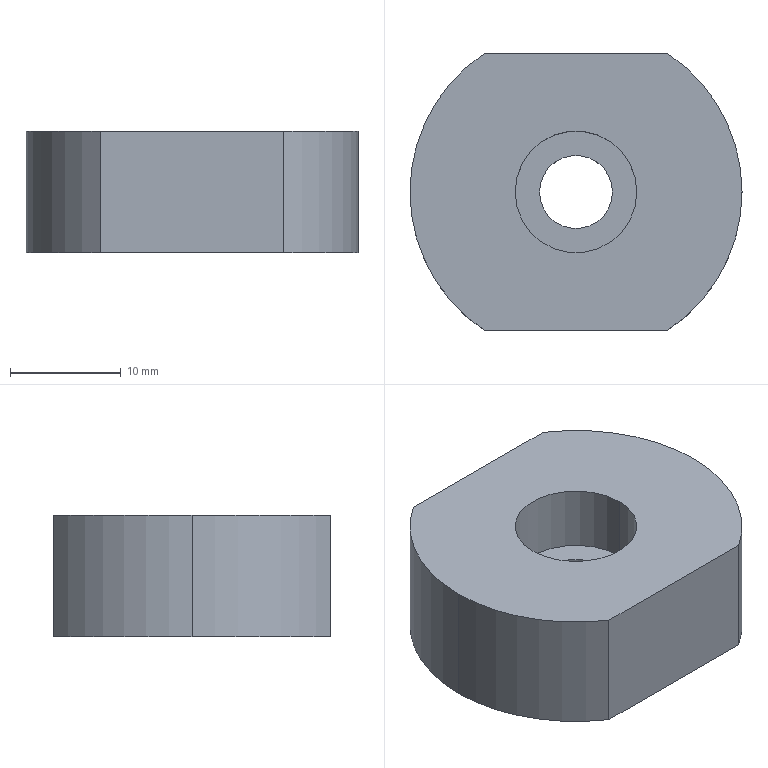Part | STEP file | union washer | 1 solid | 12 faces | box 30 x 25 x 11 mm | volume 6415 mm3 | cylinder 7 | plane 5 | commonest cylinder face diameters 30 x3 6.6 x2 11 x2
STEP:
#1=CARTESIAN_POINT('',(0.,0.,0.));
#2=DIRECTION('',(0.,0.,1.));
#3=DIRECTION('',(1.,0.,0.));
#4=AXIS2_PLACEMENT_3D('',#1,#2,#3);
#5=CARTESIAN_POINT('',(5.5,0.,5.));
#6=VERTEX_POINT('',#5);
#7=CARTESIAN_POINT('',(5.5,0.,11.));
#8=VERTEX_POINT('',#7);
#9=CARTESIAN_POINT('',(5.5,0.,11.));
#10=DIRECTION('',(0.,0.,1.));
#11=VECTOR('',#10,1.);
#12=LINE('',#9,#11);
#13=CARTESIAN_POINT('',(0.,0.,11.));
#14=DIRECTION('',(0.,0.,1.));
#15=DIRECTION('',(1.,0.,0.));
#16=AXIS2_PLACEMENT_3D('',#13,#14,#15);
#17=CYLINDRICAL_SURFACE('',#16,5.5);
#18=CARTESIAN_POINT('',(6.283,0.));
#19=DIRECTION('',(0.,1.));
#20=VECTOR('',#19,1.);
#21=LINE('',#18,#20);
#22=(GEOMETRIC_REPRESENTATION_CONTEXT(2)PARAMETRIC_REPRESENTATION_CONTEXT()REPRESENTATION_CONTEXT('',''));
#23=DEFINITIONAL_REPRESENTATION('',(#21),#22);
#24=PCURVE('',#17,#23);
#25=CARTESIAN_POINT('',(0.,0.,11.));
#26=DIRECTION('',(0.,0.,1.));
#27=DIRECTION('',(1.,0.,0.));
#28=AXIS2_PLACEMENT_3D('',#25,#26,#27);
#29=CYLINDRICAL_SURFACE('',#28,5.5);
#30=CARTESIAN_POINT('',(0.,0.));
#31=DIRECTION('',(0.,1.));
#32=VECTOR('',#31,1.);
#33=LINE('',#30,#32);
#34=(GEOMETRIC_REPRESENTATION_CONTEXT(2)PARAMETRIC_REPRESENTATION_CONTEXT()REPRESENTATION_CONTEXT('',''));
#35=DEFINITIONAL_REPRESENTATION('',(#33),#34);
#36=PCURVE('',#29,#35);
#37=SURFACE_CURVE('',#12,(#24,#36),.PCURVE_S1.);
#38=EDGE_CURVE('',#6,#8,#37,.T.);
#39=ORIENTED_EDGE('',*,*,#38,.T.);
#40=CARTESIAN_POINT('',(-5.5,0.,11.));
#41=VERTEX_POINT('',#40);
#42=CARTESIAN_POINT('',(0.,0.,11.));
#43=DIRECTION('',(0.,0.,1.));
#44=DIRECTION('',(1.,0.,0.));
#45=AXIS2_PLACEMENT_3D('',#42,#43,#44);
#46=CIRCLE('',#45,5.5);
#47=CARTESIAN_POINT('',(0.,0.));
#48=DIRECTION('',(1.,0.));
#49=VECTOR('',#48,1.);
#50=LINE('',#47,#49);
#51=(GEOMETRIC_REPRESENTATION_CONTEXT(2)PARAMETRIC_REPRESENTATION_CONTEXT()REPRESENTATION_CONTEXT('',''));
#52=DEFINITIONAL_REPRESENTATION('',(#50),#51);
#53=PCURVE('',#17,#52);
#54=CARTESIAN_POINT('',(0.,0.,11.));
#55=DIRECTION('',(0.,0.,1.));
#56=DIRECTION('',(1.,0.,0.));
#57=AXIS2_PLACEMENT_3D('',#54,#55,#56);
#58=PLANE('',#57);
#59=CARTESIAN_POINT('',(0.,0.));
#60=DIRECTION('',(1.,0.));
#61=AXIS2_PLACEMENT_2D('',#59,#60);
#62=CIRCLE('',#61,5.5);
#63=(GEOMETRIC_REPRESENTATION_CONTEXT(2)PARAMETRIC_REPRESENTATION_CONTEXT()REPRESENTATION_CONTEXT('',''));
#64=DEFINITIONAL_REPRESENTATION('',(#62),#63);
#65=PCURVE('',#58,#64);
#66=SURFACE_CURVE('',#46,(#53,#65),.PCURVE_S1.);
#67=EDGE_CURVE('',#41,#8,#66,.T.);
#68=ORIENTED_EDGE('',*,*,#67,.F.);
#69=CARTESIAN_POINT('',(-5.5,0.,5.));
#70=VERTEX_POINT('',#69);
#71=CARTESIAN_POINT('',(-5.5,0.,11.));
#72=DIRECTION('',(0.,0.,1.));
#73=VECTOR('',#72,1.);
#74=LINE('',#71,#73);
#75=CARTESIAN_POINT('',(3.142,0.));
#76=DIRECTION('',(0.,1.));
#77=VECTOR('',#76,1.);
#78=LINE('',#75,#77);
#79=(GEOMETRIC_REPRESENTATION_CONTEXT(2)PARAMETRIC_REPRESENTATION_CONTEXT()REPRESENTATION_CONTEXT('',''));
#80=DEFINITIONAL_REPRESENTATION('',(#78),#79);
#81=PCURVE('',#17,#80);
#82=CARTESIAN_POINT('',(3.142,0.));
#83=DIRECTION('',(0.,1.));
#84=VECTOR('',#83,1.);
#85=LINE('',#82,#84);
#86=(GEOMETRIC_REPRESENTATION_CONTEXT(2)PARAMETRIC_REPRESENTATION_CONTEXT()REPRESENTATION_CONTEXT('',''));
#87=DEFINITIONAL_REPRESENTATION('',(#85),#86);
#88=PCURVE('',#29,#87);
#89=SURFACE_CURVE('',#74,(#81,#88),.PCURVE_S1.);
#90=EDGE_CURVE('',#70,#41,#89,.T.);
#91=ORIENTED_EDGE('',*,*,#90,.F.);
#92=CARTESIAN_POINT('',(0.,0.,5.));
#93=DIRECTION('',(0.,0.,1.));
#94=DIRECTION('',(1.,0.,0.));
#95=AXIS2_PLACEMENT_3D('',#92,#93,#94);
#96=CIRCLE('',#95,5.5);
#97=CARTESIAN_POINT('',(0.,-6.));
#98=DIRECTION('',(1.,0.));
#99=VECTOR('',#98,1.);
#100=LINE('',#97,#99);
#101=(GEOMETRIC_REPRESENTATION_CONTEXT(2)PARAMETRIC_REPRESENTATION_CONTEXT()REPRESENTATION_CONTEXT('',''));
#102=DEFINITIONAL_REPRESENTATION('',(#100),#101);
#103=PCURVE('',#17,#102);
#104=CARTESIAN_POINT('',(3.3,0.,5.));
#105=DIRECTION('',(0.,0.,-1.));
#106=DIRECTION('',(-1.,0.,0.));
#107=AXIS2_PLACEMENT_3D('',#104,#105,#106);
#108=PLANE('',#107);
#109=CARTESIAN_POINT('',(-2.2,0.));
#110=CARTESIAN_POINT('',(-2.2,9.526));
#111=CARTESIAN_POINT('',(6.05,4.763));
#112=CARTESIAN_POINT('',(14.3,0.));
#113=CARTESIAN_POINT('',(6.05,-4.763));
#114=CARTESIAN_POINT('',(-2.2,-9.526));
#115=CARTESIAN_POINT('',(-2.2,0.));
#116=(BOUNDED_CURVE()B_SPLINE_CURVE(2,(#109,#110,#111,#112,#113,#114,#115),.UNSPECIFIED.,.T.,.F.)B_SPLINE_CURVE_WITH_KNOTS((1,2,2,2,2,1),(-2.094,0.,2.094,4.189,6.283,8.378),.UNSPECIFIED.)CURVE()GEOMETRIC_REPRESENTATION_ITEM()RATIONAL_B_SPLINE_CURVE((1.,0.5,1.,0.5,1.,0.5,1.))REPRESENTATION_ITEM(''));
#117=(GEOMETRIC_REPRESENTATION_CONTEXT(2)PARAMETRIC_REPRESENTATION_CONTEXT()REPRESENTATION_CONTEXT('',''));
#118=DEFINITIONAL_REPRESENTATION('',(#116),#117);
#119=PCURVE('',#108,#118);
#120=SURFACE_CURVE('',#96,(#103,#119),.PCURVE_S1.);
#121=EDGE_CURVE('',#70,#6,#120,.T.);
#122=ORIENTED_EDGE('',*,*,#121,.T.);
#123=EDGE_LOOP('',(#39,#68,#91,#122));
#124=FACE_BOUND('',#123,.F.);
#125=ADVANCED_FACE('',(#124),#17,.F.);
#126=CARTESIAN_POINT('',(-3.3,0.,5.));
#127=VERTEX_POINT('',#126);
#128=CARTESIAN_POINT('',(-3.3,0.,0.));
#129=VERTEX_POINT('',#128);
#130=CARTESIAN_POINT('',(-3.3,0.,11.));
#131=DIRECTION('',(0.,0.,-1.));
#132=VECTOR('',#131,1.);
#133=LINE('',#130,#132);
#134=CARTESIAN_POINT('',(0.,0.,11.));
#135=DIRECTION('',(0.,0.,-1.));
#136=DIRECTION('',(-1.,0.,0.));
#137=AXIS2_PLACEMENT_3D('',#134,#135,#136);
#138=CYLINDRICAL_SURFACE('',#137,3.3);
#139=CARTESIAN_POINT('',(6.283,0.));
#140=DIRECTION('',(0.,1.));
#141=VECTOR('',#140,1.);
#142=LINE('',#139,#141);
#143=(GEOMETRIC_REPRESENTATION_CONTEXT(2)PARAMETRIC_REPRESENTATION_CONTEXT()REPRESENTATION_CONTEXT('',''));
#144=DEFINITIONAL_REPRESENTATION('',(#142),#143);
#145=PCURVE('',#138,#144);
#146=CARTESIAN_POINT('',(0.,0.,11.));
#147=DIRECTION('',(0.,0.,-1.));
#148=DIRECTION('',(-1.,0.,0.));
#149=AXIS2_PLACEMENT_3D('',#146,#147,#148);
#150=CYLINDRICAL_SURFACE('',#149,3.3);
#151=CARTESIAN_POINT('',(0.,0.));
#152=DIRECTION('',(0.,1.));
#153=VECTOR('',#152,1.);
#154=LINE('',#151,#153);
#155=(GEOMETRIC_REPRESENTATION_CONTEXT(2)PARAMETRIC_REPRESENTATION_CONTEXT()REPRESENTATION_CONTEXT('',''));
#156=DEFINITIONAL_REPRESENTATION('',(#154),#155);
#157=PCURVE('',#150,#156);
#158=SURFACE_CURVE('',#133,(#145,#157),.PCURVE_S1.);
#159=EDGE_CURVE('',#127,#129,#158,.T.);
#160=ORIENTED_EDGE('',*,*,#159,.T.);
#161=CARTESIAN_POINT('',(3.3,0.,0.));
#162=VERTEX_POINT('',#161);
#163=CARTESIAN_POINT('',(0.,0.,0.));
#164=DIRECTION('',(0.,0.,1.));
#165=DIRECTION('',(1.,0.,0.));
#166=AXIS2_PLACEMENT_3D('',#163,#164,#165);
#167=CIRCLE('',#166,3.3);
#168=CARTESIAN_POINT('',(9.425,11.));
#169=DIRECTION('',(-1.,0.));
#170=VECTOR('',#169,1.);
#171=LINE('',#168,#170);
#172=(GEOMETRIC_REPRESENTATION_CONTEXT(2)PARAMETRIC_REPRESENTATION_CONTEXT()REPRESENTATION_CONTEXT('',''));
#173=DEFINITIONAL_REPRESENTATION('',(#171),#172);
#174=PCURVE('',#138,#173);
#175=CARTESIAN_POINT('',(0.,0.,0.));
#176=DIRECTION('',(0.,0.,1.));
#177=DIRECTION('',(1.,0.,0.));
#178=AXIS2_PLACEMENT_3D('',#175,#176,#177);
#179=PLANE('',#178);
#180=CARTESIAN_POINT('',(0.,0.));
#181=DIRECTION('',(1.,0.));
#182=AXIS2_PLACEMENT_2D('',#180,#181);
#183=CIRCLE('',#182,3.3);
#184=(GEOMETRIC_REPRESENTATION_CONTEXT(2)PARAMETRIC_REPRESENTATION_CONTEXT()REPRESENTATION_CONTEXT('',''));
#185=DEFINITIONAL_REPRESENTATION('',(#183),#184);
#186=PCURVE('',#179,#185);
#187=SURFACE_CURVE('',#167,(#174,#186),.PCURVE_S1.);
#188=EDGE_CURVE('',#129,#162,#187,.T.);
#189=ORIENTED_EDGE('',*,*,#188,.T.);
#190=CARTESIAN_POINT('',(3.3,0.,5.));
#191=VERTEX_POINT('',#190);
#192=CARTESIAN_POINT('',(3.3,0.,11.));
#193=DIRECTION('',(0.,0.,-1.));
#194=VECTOR('',#193,1.);
#195=LINE('',#192,#194);
#196=CARTESIAN_POINT('',(3.142,0.));
#197=DIRECTION('',(0.,1.));
#198=VECTOR('',#197,1.);
#199=LINE('',#196,#198);
#200=(GEOMETRIC_REPRESENTATION_CONTEXT(2)PARAMETRIC_REPRESENTATION_CONTEXT()REPRESENTATION_CONTEXT('',''));
#201=DEFINITIONAL_REPRESENTATION('',(#199),#200);
#202=PCURVE('',#138,#201);
#203=CARTESIAN_POINT('',(3.142,0.));
#204=DIRECTION('',(0.,1.));
#205=VECTOR('',#204,1.);
#206=LINE('',#203,#205);
#207=(GEOMETRIC_REPRESENTATION_CONTEXT(2)PARAMETRIC_REPRESENTATION_CONTEXT()REPRESENTATION_CONTEXT('',''));
#208=DEFINITIONAL_REPRESENTATION('',(#206),#207);
#209=PCURVE('',#150,#208);
#210=SURFACE_CURVE('',#195,(#202,#209),.PCURVE_S1.);
#211=EDGE_CURVE('',#191,#162,#210,.T.);
#212=ORIENTED_EDGE('',*,*,#211,.F.);
#213=CARTESIAN_POINT('',(0.,0.,5.));
#214=DIRECTION('',(0.,0.,1.));
#215=DIRECTION('',(1.,0.,0.));
#216=AXIS2_PLACEMENT_3D('',#213,#214,#215);
#217=CIRCLE('',#216,3.3);
#218=CARTESIAN_POINT('',(9.425,6.));
#219=DIRECTION('',(-1.,0.));
#220=VECTOR('',#219,1.);
#221=LINE('',#218,#220);
#222=(GEOMETRIC_REPRESENTATION_CONTEXT(2)PARAMETRIC_REPRESENTATION_CONTEXT()REPRESENTATION_CONTEXT('',''));
#223=DEFINITIONAL_REPRESENTATION('',(#221),#222);
#224=PCURVE('',#138,#223);
#225=CARTESIAN_POINT('',(0.,0.));
#226=CARTESIAN_POINT('',(0.,5.716));
#227=CARTESIAN_POINT('',(4.95,2.858));
#228=CARTESIAN_POINT('',(9.9,0.));
#229=CARTESIAN_POINT('',(4.95,-2.858));
#230=CARTESIAN_POINT('',(0.,-5.716));
#231=CARTESIAN_POINT('',(0.,0.));
#232=(BOUNDED_CURVE()B_SPLINE_CURVE(2,(#225,#226,#227,#228,#229,#230,#231),.UNSPECIFIED.,.T.,.F.)B_SPLINE_CURVE_WITH_KNOTS((1,2,2,2,2,1),(-2.094,0.,2.094,4.189,6.283,8.378),.UNSPECIFIED.)CURVE()GEOMETRIC_REPRESENTATION_ITEM()RATIONAL_B_SPLINE_CURVE((1.,0.5,1.,0.5,1.,0.5,1.))REPRESENTATION_ITEM(''));
#233=(GEOMETRIC_REPRESENTATION_CONTEXT(2)PARAMETRIC_REPRESENTATION_CONTEXT()REPRESENTATION_CONTEXT('',''));
#234=DEFINITIONAL_REPRESENTATION('',(#232),#233);
#235=PCURVE('',#108,#234);
#236=SURFACE_CURVE('',#217,(#224,#235),.PCURVE_S1.);
#237=EDGE_CURVE('',#127,#191,#236,.T.);
#238=ORIENTED_EDGE('',*,*,#237,.F.);
#239=EDGE_LOOP('',(#160,#189,#212,#238));
#240=FACE_BOUND('',#239,.F.);
#241=ADVANCED_FACE('',(#240),#138,.F.);
#242=CARTESIAN_POINT('',(-15.,0.,11.));
#243=VERTEX_POINT('',#242);
#244=CARTESIAN_POINT('',(-8.292,-12.5,11.));
#245=VERTEX_POINT('',#244);
#246=CARTESIAN_POINT('',(0.,0.,11.));
#247=DIRECTION('',(0.,0.,1.));
#248=DIRECTION('',(1.,0.,0.));
#249=AXIS2_PLACEMENT_3D('',#246,#247,#248);
#250=CIRCLE('',#249,15.);
#251=CARTESIAN_POINT('',(0.,0.,11.));
#252=DIRECTION('',(0.,0.,-1.));
#253=DIRECTION('',(-1.,0.,0.));
#254=AXIS2_PLACEMENT_3D('',#251,#252,#253);
#255=CYLINDRICAL_SURFACE('',#254,15.);
#256=CARTESIAN_POINT('',(9.425,0.));
#257=DIRECTION('',(-1.,0.));
#258=VECTOR('',#257,1.);
#259=LINE('',#256,#258);
#260=(GEOMETRIC_REPRESENTATION_CONTEXT(2)PARAMETRIC_REPRESENTATION_CONTEXT()REPRESENTATION_CONTEXT('',''));
#261=DEFINITIONAL_REPRESENTATION('',(#259),#260);
#262=PCURVE('',#255,#261);
#263=CARTESIAN_POINT('',(0.,0.));
#264=DIRECTION('',(1.,0.));
#265=AXIS2_PLACEMENT_2D('',#263,#264);
#266=CIRCLE('',#265,15.);
#267=(GEOMETRIC_REPRESENTATION_CONTEXT(2)PARAMETRIC_REPRESENTATION_CONTEXT()REPRESENTATION_CONTEXT('',''));
#268=DEFINITIONAL_REPRESENTATION('',(#266),#267);
#269=PCURVE('',#58,#268);
#270=SURFACE_CURVE('',#250,(#262,#269),.PCURVE_S1.);
#271=EDGE_CURVE('',#243,#245,#270,.T.);
#272=ORIENTED_EDGE('',*,*,#271,.F.);
#273=CARTESIAN_POINT('',(-15.,0.,0.));
#274=VERTEX_POINT('',#273);
#275=CARTESIAN_POINT('',(-15.,0.,11.));
#276=DIRECTION('',(0.,0.,-1.));
#277=VECTOR('',#276,1.);
#278=LINE('',#275,#277);
#279=CARTESIAN_POINT('',(6.283,0.));
#280=DIRECTION('',(0.,1.));
#281=VECTOR('',#280,1.);
#282=LINE('',#279,#281);
#283=(GEOMETRIC_REPRESENTATION_CONTEXT(2)PARAMETRIC_REPRESENTATION_CONTEXT()REPRESENTATION_CONTEXT('',''));
#284=DEFINITIONAL_REPRESENTATION('',(#282),#283);
#285=PCURVE('',#255,#284);
#286=CARTESIAN_POINT('',(0.,0.,11.));
#287=DIRECTION('',(0.,0.,-1.));
#288=DIRECTION('',(-1.,0.,0.));
#289=AXIS2_PLACEMENT_3D('',#286,#287,#288);
#290=CYLINDRICAL_SURFACE('',#289,15.);
#291=CARTESIAN_POINT('',(0.,0.));
#292=DIRECTION('',(0.,1.));
#293=VECTOR('',#292,1.);
#294=LINE('',#291,#293);
#295=(GEOMETRIC_REPRESENTATION_CONTEXT(2)PARAMETRIC_REPRESENTATION_CONTEXT()REPRESENTATION_CONTEXT('',''));
#296=DEFINITIONAL_REPRESENTATION('',(#294),#295);
#297=PCURVE('',#290,#296);
#298=SURFACE_CURVE('',#278,(#285,#297),.PCURVE_S1.);
#299=EDGE_CURVE('',#243,#274,#298,.T.);
#300=ORIENTED_EDGE('',*,*,#299,.T.);
#301=CARTESIAN_POINT('',(-8.292,-12.5,0.));
#302=VERTEX_POINT('',#301);
#303=CARTESIAN_POINT('',(0.,0.,0.));
#304=DIRECTION('',(0.,0.,1.));
#305=DIRECTION('',(1.,0.,0.));
#306=AXIS2_PLACEMENT_3D('',#303,#304,#305);
#307=CIRCLE('',#306,15.);
#308=CARTESIAN_POINT('',(9.425,11.));
#309=DIRECTION('',(-1.,0.));
#310=VECTOR('',#309,1.);
#311=LINE('',#308,#310);
#312=(GEOMETRIC_REPRESENTATION_CONTEXT(2)PARAMETRIC_REPRESENTATION_CONTEXT()REPRESENTATION_CONTEXT('',''));
#313=DEFINITIONAL_REPRESENTATION('',(#311),#312);
#314=PCURVE('',#255,#313);
#315=CARTESIAN_POINT('',(0.,0.));
#316=DIRECTION('',(1.,0.));
#317=AXIS2_PLACEMENT_2D('',#315,#316);
#318=CIRCLE('',#317,15.);
#319=(GEOMETRIC_REPRESENTATION_CONTEXT(2)PARAMETRIC_REPRESENTATION_CONTEXT()REPRESENTATION_CONTEXT('',''));
#320=DEFINITIONAL_REPRESENTATION('',(#318),#319);
#321=PCURVE('',#179,#320);
#322=SURFACE_CURVE('',#307,(#314,#321),.PCURVE_S1.);
#323=EDGE_CURVE('',#274,#302,#322,.T.);
#324=ORIENTED_EDGE('',*,*,#323,.T.);
#325=CARTESIAN_POINT('',(-8.292,-12.5,11.));
#326=DIRECTION('',(0.,0.,-1.));
#327=VECTOR('',#326,1.);
#328=LINE('',#325,#327);
#329=CARTESIAN_POINT('',(5.298,0.));
#330=DIRECTION('',(0.,1.));
#331=VECTOR('',#330,1.);
#332=LINE('',#329,#331);
#333=(GEOMETRIC_REPRESENTATION_CONTEXT(2)PARAMETRIC_REPRESENTATION_CONTEXT()REPRESENTATION_CONTEXT('',''));
#334=DEFINITIONAL_REPRESENTATION('',(#332),#333);
#335=PCURVE('',#255,#334);
#336=CARTESIAN_POINT('',(-8.292,-12.5,11.));
#337=DIRECTION('',(0.,1.,0.));
#338=DIRECTION('',(0.,0.,1.));
#339=AXIS2_PLACEMENT_3D('',#336,#337,#338);
#340=PLANE('',#339);
#341=CARTESIAN_POINT('',(0.,0.));
#342=DIRECTION('',(-1.,0.));
#343=VECTOR('',#342,1.);
#344=LINE('',#341,#343);
#345=(GEOMETRIC_REPRESENTATION_CONTEXT(2)PARAMETRIC_REPRESENTATION_CONTEXT()REPRESENTATION_CONTEXT('',''));
#346=DEFINITIONAL_REPRESENTATION('',(#344),#345);
#347=PCURVE('',#340,#346);
#348=SURFACE_CURVE('',#328,(#335,#347),.PCURVE_S1.);
#349=EDGE_CURVE('',#245,#302,#348,.T.);
#350=ORIENTED_EDGE('',*,*,#349,.F.);
#351=EDGE_LOOP('',(#272,#300,#324,#350));
#352=FACE_BOUND('',#351,.T.);
#353=ADVANCED_FACE('',(#352),#255,.T.);
#354=CARTESIAN_POINT('',(0.,0.,11.));
#355=DIRECTION('',(0.,0.,1.));
#356=DIRECTION('',(1.,0.,0.));
#357=AXIS2_PLACEMENT_3D('',#354,#355,#356);
#358=CIRCLE('',#357,5.5);
#359=CARTESIAN_POINT('',(0.,0.));
#360=DIRECTION('',(1.,0.));
#361=AXIS2_PLACEMENT_2D('',#359,#360);
#362=CIRCLE('',#361,5.5);
#363=(GEOMETRIC_REPRESENTATION_CONTEXT(2)PARAMETRIC_REPRESENTATION_CONTEXT()REPRESENTATION_CONTEXT('',''));
#364=DEFINITIONAL_REPRESENTATION('',(#362),#363);
#365=PCURVE('',#58,#364);
#366=CARTESIAN_POINT('',(0.,0.));
#367=DIRECTION('',(1.,0.));
#368=VECTOR('',#367,1.);
#369=LINE('',#366,#368);
#370=(GEOMETRIC_REPRESENTATION_CONTEXT(2)PARAMETRIC_REPRESENTATION_CONTEXT()REPRESENTATION_CONTEXT('',''));
#371=DEFINITIONAL_REPRESENTATION('',(#369),#370);
#372=PCURVE('',#29,#371);
#373=SURFACE_CURVE('',#358,(#365,#372),.PCURVE_S1.);
#374=EDGE_CURVE('',#8,#41,#373,.T.);
#375=ORIENTED_EDGE('',*,*,#374,.F.);
#376=ORIENTED_EDGE('',*,*,#67,.F.);
#377=EDGE_LOOP('',(#375,#376));
#378=FACE_BOUND('',#377,.T.);
#379=CARTESIAN_POINT('',(-8.292,12.5,11.));
#380=VERTEX_POINT('',#379);
#381=CARTESIAN_POINT('',(0.,0.,11.));
#382=DIRECTION('',(0.,0.,1.));
#383=DIRECTION('',(1.,0.,0.));
#384=AXIS2_PLACEMENT_3D('',#381,#382,#383);
#385=CIRCLE('',#384,15.);
#386=CARTESIAN_POINT('',(0.,0.));
#387=DIRECTION('',(1.,0.));
#388=AXIS2_PLACEMENT_2D('',#386,#387);
#389=CIRCLE('',#388,15.);
#390=(GEOMETRIC_REPRESENTATION_CONTEXT(2)PARAMETRIC_REPRESENTATION_CONTEXT()REPRESENTATION_CONTEXT('',''));
#391=DEFINITIONAL_REPRESENTATION('',(#389),#390);
#392=PCURVE('',#58,#391);
#393=CARTESIAN_POINT('',(3.142,0.));
#394=DIRECTION('',(-1.,0.));
#395=VECTOR('',#394,1.);
#396=LINE('',#393,#395);
#397=(GEOMETRIC_REPRESENTATION_CONTEXT(2)PARAMETRIC_REPRESENTATION_CONTEXT()REPRESENTATION_CONTEXT('',''));
#398=DEFINITIONAL_REPRESENTATION('',(#396),#397);
#399=PCURVE('',#290,#398);
#400=SURFACE_CURVE('',#385,(#392,#399),.PCURVE_S1.);
#401=EDGE_CURVE('',#380,#243,#400,.T.);
#402=ORIENTED_EDGE('',*,*,#401,.T.);
#403=ORIENTED_EDGE('',*,*,#271,.T.);
#404=CARTESIAN_POINT('',(8.292,-12.5,11.));
#405=VERTEX_POINT('',#404);
#406=CARTESIAN_POINT('',(-8.292,-12.5,11.));
#407=DIRECTION('',(1.,0.,0.));
#408=VECTOR('',#407,1.);
#409=LINE('',#406,#408);
#410=CARTESIAN_POINT('',(-8.292,-12.5));
#411=DIRECTION('',(1.,0.));
#412=VECTOR('',#411,1.);
#413=LINE('',#410,#412);
#414=(GEOMETRIC_REPRESENTATION_CONTEXT(2)PARAMETRIC_REPRESENTATION_CONTEXT()REPRESENTATION_CONTEXT('',''));
#415=DEFINITIONAL_REPRESENTATION('',(#413),#414);
#416=PCURVE('',#58,#415);
#417=CARTESIAN_POINT('',(0.,0.));
#418=DIRECTION('',(0.,1.));
#419=VECTOR('',#418,1.);
#420=LINE('',#417,#419);
#421=(GEOMETRIC_REPRESENTATION_CONTEXT(2)PARAMETRIC_REPRESENTATION_CONTEXT()REPRESENTATION_CONTEXT('',''));
#422=DEFINITIONAL_REPRESENTATION('',(#420),#421);
#423=PCURVE('',#340,#422);
#424=SURFACE_CURVE('',#409,(#416,#423),.PCURVE_S1.);
#425=EDGE_CURVE('',#245,#405,#424,.T.);
#426=ORIENTED_EDGE('',*,*,#425,.T.);
#427=CARTESIAN_POINT('',(8.292,12.5,11.));
#428=VERTEX_POINT('',#427);
#429=CARTESIAN_POINT('',(0.,0.,11.));
#430=DIRECTION('',(0.,0.,1.));
#431=DIRECTION('',(1.,0.,0.));
#432=AXIS2_PLACEMENT_3D('',#429,#430,#431);
#433=CIRCLE('',#432,15.);
#434=CARTESIAN_POINT('',(0.,0.));
#435=DIRECTION('',(1.,0.));
#436=AXIS2_PLACEMENT_2D('',#434,#435);
#437=CIRCLE('',#436,15.);
#438=(GEOMETRIC_REPRESENTATION_CONTEXT(2)PARAMETRIC_REPRESENTATION_CONTEXT()REPRESENTATION_CONTEXT('',''));
#439=DEFINITIONAL_REPRESENTATION('',(#437),#438);
#440=PCURVE('',#58,#439);
#441=CARTESIAN_POINT('',(0.,0.,11.));
#442=DIRECTION('',(0.,0.,-1.));
#443=DIRECTION('',(-1.,0.,0.));
#444=AXIS2_PLACEMENT_3D('',#441,#442,#443);
#445=CYLINDRICAL_SURFACE('',#444,15.);
#446=CARTESIAN_POINT('',(9.425,0.));
#447=DIRECTION('',(-1.,0.));
#448=VECTOR('',#447,1.);
#449=LINE('',#446,#448);
#450=(GEOMETRIC_REPRESENTATION_CONTEXT(2)PARAMETRIC_REPRESENTATION_CONTEXT()REPRESENTATION_CONTEXT('',''));
#451=DEFINITIONAL_REPRESENTATION('',(#449),#450);
#452=PCURVE('',#445,#451);
#453=SURFACE_CURVE('',#433,(#440,#452),.PCURVE_S1.);
#454=EDGE_CURVE('',#405,#428,#453,.T.);
#455=ORIENTED_EDGE('',*,*,#454,.T.);
#456=CARTESIAN_POINT('',(8.292,12.5,11.));
#457=DIRECTION('',(-1.,0.,0.));
#458=VECTOR('',#457,1.);
#459=LINE('',#456,#458);
#460=CARTESIAN_POINT('',(8.292,12.5));
#461=DIRECTION('',(-1.,0.));
#462=VECTOR('',#461,1.);
#463=LINE('',#460,#462);
#464=(GEOMETRIC_REPRESENTATION_CONTEXT(2)PARAMETRIC_REPRESENTATION_CONTEXT()REPRESENTATION_CONTEXT('',''));
#465=DEFINITIONAL_REPRESENTATION('',(#463),#464);
#466=PCURVE('',#58,#465);
#467=CARTESIAN_POINT('',(8.292,12.5,11.));
#468=DIRECTION('',(0.,-1.,0.));
#469=DIRECTION('',(0.,0.,-1.));
#470=AXIS2_PLACEMENT_3D('',#467,#468,#469);
#471=PLANE('',#470);
#472=CARTESIAN_POINT('',(0.,0.));
#473=DIRECTION('',(0.,-1.));
#474=VECTOR('',#473,1.);
#475=LINE('',#472,#474);
#476=(GEOMETRIC_REPRESENTATION_CONTEXT(2)PARAMETRIC_REPRESENTATION_CONTEXT()REPRESENTATION_CONTEXT('',''));
#477=DEFINITIONAL_REPRESENTATION('',(#475),#476);
#478=PCURVE('',#471,#477);
#479=SURFACE_CURVE('',#459,(#466,#478),.PCURVE_S1.);
#480=EDGE_CURVE('',#428,#380,#479,.T.);
#481=ORIENTED_EDGE('',*,*,#480,.T.);
#482=EDGE_LOOP('',(#402,#403,#426,#455,#481));
#483=FACE_BOUND('',#482,.T.);
#484=ADVANCED_FACE('',(#378,#483),#58,.T.);
#485=CARTESIAN_POINT('',(-8.292,12.5,0.));
#486=VERTEX_POINT('',#485);
#487=CARTESIAN_POINT('',(0.,0.,0.));
#488=DIRECTION('',(0.,0.,1.));
#489=DIRECTION('',(1.,0.,0.));
#490=AXIS2_PLACEMENT_3D('',#487,#488,#489);
#491=CIRCLE('',#490,15.);
#492=CARTESIAN_POINT('',(0.,0.));
#493=DIRECTION('',(1.,0.));
#494=AXIS2_PLACEMENT_2D('',#492,#493);
#495=CIRCLE('',#494,15.);
#496=(GEOMETRIC_REPRESENTATION_CONTEXT(2)PARAMETRIC_REPRESENTATION_CONTEXT()REPRESENTATION_CONTEXT('',''));
#497=DEFINITIONAL_REPRESENTATION('',(#495),#496);
#498=PCURVE('',#179,#497);
#499=CARTESIAN_POINT('',(3.142,11.));
#500=DIRECTION('',(-1.,0.));
#501=VECTOR('',#500,1.);
#502=LINE('',#499,#501);
#503=(GEOMETRIC_REPRESENTATION_CONTEXT(2)PARAMETRIC_REPRESENTATION_CONTEXT()REPRESENTATION_CONTEXT('',''));
#504=DEFINITIONAL_REPRESENTATION('',(#502),#503);
#505=PCURVE('',#290,#504);
#506=SURFACE_CURVE('',#491,(#498,#505),.PCURVE_S1.);
#507=EDGE_CURVE('',#486,#274,#506,.T.);
#508=ORIENTED_EDGE('',*,*,#507,.F.);
#509=CARTESIAN_POINT('',(8.292,12.5,0.));
#510=VERTEX_POINT('',#509);
#511=CARTESIAN_POINT('',(8.292,12.5,0.));
#512=DIRECTION('',(-1.,0.,0.));
#513=VECTOR('',#512,1.);
#514=LINE('',#511,#513);
#515=CARTESIAN_POINT('',(8.292,12.5));
#516=DIRECTION('',(-1.,0.));
#517=VECTOR('',#516,1.);
#518=LINE('',#515,#517);
#519=(GEOMETRIC_REPRESENTATION_CONTEXT(2)PARAMETRIC_REPRESENTATION_CONTEXT()REPRESENTATION_CONTEXT('',''));
#520=DEFINITIONAL_REPRESENTATION('',(#518),#519);
#521=PCURVE('',#179,#520);
#522=CARTESIAN_POINT('',(11.,0.));
#523=DIRECTION('',(0.,-1.));
#524=VECTOR('',#523,1.);
#525=LINE('',#522,#524);
#526=(GEOMETRIC_REPRESENTATION_CONTEXT(2)PARAMETRIC_REPRESENTATION_CONTEXT()REPRESENTATION_CONTEXT('',''));
#527=DEFINITIONAL_REPRESENTATION('',(#525),#526);
#528=PCURVE('',#471,#527);
#529=SURFACE_CURVE('',#514,(#521,#528),.PCURVE_S1.);
#530=EDGE_CURVE('',#510,#486,#529,.T.);
#531=ORIENTED_EDGE('',*,*,#530,.F.);
#532=CARTESIAN_POINT('',(8.292,-12.5,0.));
#533=VERTEX_POINT('',#532);
#534=CARTESIAN_POINT('',(0.,0.,0.));
#535=DIRECTION('',(0.,0.,1.));
#536=DIRECTION('',(1.,0.,0.));
#537=AXIS2_PLACEMENT_3D('',#534,#535,#536);
#538=CIRCLE('',#537,15.);
#539=CARTESIAN_POINT('',(0.,0.));
#540=DIRECTION('',(1.,0.));
#541=AXIS2_PLACEMENT_2D('',#539,#540);
#542=CIRCLE('',#541,15.);
#543=(GEOMETRIC_REPRESENTATION_CONTEXT(2)PARAMETRIC_REPRESENTATION_CONTEXT()REPRESENTATION_CONTEXT('',''));
#544=DEFINITIONAL_REPRESENTATION('',(#542),#543);
#545=PCURVE('',#179,#544);
#546=CARTESIAN_POINT('',(9.425,11.));
#547=DIRECTION('',(-1.,0.));
#548=VECTOR('',#547,1.);
#549=LINE('',#546,#548);
#550=(GEOMETRIC_REPRESENTATION_CONTEXT(2)PARAMETRIC_REPRESENTATION_CONTEXT()REPRESENTATION_CONTEXT('',''));
#551=DEFINITIONAL_REPRESENTATION('',(#549),#550);
#552=PCURVE('',#445,#551);
#553=SURFACE_CURVE('',#538,(#545,#552),.PCURVE_S1.);
#554=EDGE_CURVE('',#533,#510,#553,.T.);
#555=ORIENTED_EDGE('',*,*,#554,.F.);
#556=CARTESIAN_POINT('',(-8.292,-12.5,0.));
#557=DIRECTION('',(1.,0.,0.));
#558=VECTOR('',#557,1.);
#559=LINE('',#556,#558);
#560=CARTESIAN_POINT('',(-8.292,-12.5));
#561=DIRECTION('',(1.,0.));
#562=VECTOR('',#561,1.);
#563=LINE('',#560,#562);
#564=(GEOMETRIC_REPRESENTATION_CONTEXT(2)PARAMETRIC_REPRESENTATION_CONTEXT()REPRESENTATION_CONTEXT('',''));
#565=DEFINITIONAL_REPRESENTATION('',(#563),#564);
#566=PCURVE('',#179,#565);
#567=CARTESIAN_POINT('',(-11.,0.));
#568=DIRECTION('',(0.,1.));
#569=VECTOR('',#568,1.);
#570=LINE('',#567,#569);
#571=(GEOMETRIC_REPRESENTATION_CONTEXT(2)PARAMETRIC_REPRESENTATION_CONTEXT()REPRESENTATION_CONTEXT('',''));
#572=DEFINITIONAL_REPRESENTATION('',(#570),#571);
#573=PCURVE('',#340,#572);
#574=SURFACE_CURVE('',#559,(#566,#573),.PCURVE_S1.);
#575=EDGE_CURVE('',#302,#533,#574,.T.);
#576=ORIENTED_EDGE('',*,*,#575,.F.);
#577=ORIENTED_EDGE('',*,*,#323,.F.);
#578=EDGE_LOOP('',(#508,#531,#555,#576,#577));
#579=FACE_BOUND('',#578,.T.);
#580=ORIENTED_EDGE('',*,*,#188,.T.);
#581=CARTESIAN_POINT('',(0.,0.,0.));
#582=DIRECTION('',(0.,0.,1.));
#583=DIRECTION('',(1.,0.,0.));
#584=AXIS2_PLACEMENT_3D('',#581,#582,#583);
#585=CIRCLE('',#584,3.3);
#586=CARTESIAN_POINT('',(0.,0.));
#587=DIRECTION('',(1.,0.));
#588=AXIS2_PLACEMENT_2D('',#586,#587);
#589=CIRCLE('',#588,3.3);
#590=(GEOMETRIC_REPRESENTATION_CONTEXT(2)PARAMETRIC_REPRESENTATION_CONTEXT()REPRESENTATION_CONTEXT('',''));
#591=DEFINITIONAL_REPRESENTATION('',(#589),#590);
#592=PCURVE('',#179,#591);
#593=CARTESIAN_POINT('',(3.142,11.));
#594=DIRECTION('',(-1.,0.));
#595=VECTOR('',#594,1.);
#596=LINE('',#593,#595);
#597=(GEOMETRIC_REPRESENTATION_CONTEXT(2)PARAMETRIC_REPRESENTATION_CONTEXT()REPRESENTATION_CONTEXT('',''));
#598=DEFINITIONAL_REPRESENTATION('',(#596),#597);
#599=PCURVE('',#150,#598);
#600=SURFACE_CURVE('',#585,(#592,#599),.PCURVE_S1.);
#601=EDGE_CURVE('',#162,#129,#600,.T.);
#602=ORIENTED_EDGE('',*,*,#601,.T.);
#603=EDGE_LOOP('',(#580,#602));
#604=FACE_BOUND('',#603,.T.);
#605=ADVANCED_FACE('',(#579,#604),#179,.F.);
#606=ORIENTED_EDGE('',*,*,#299,.F.);
#607=ORIENTED_EDGE('',*,*,#401,.F.);
#608=CARTESIAN_POINT('',(-8.292,12.5,11.));
#609=DIRECTION('',(0.,0.,-1.));
#610=VECTOR('',#609,1.);
#611=LINE('',#608,#610);
#612=CARTESIAN_POINT('',(0.9851,0.));
#613=DIRECTION('',(0.,1.));
#614=VECTOR('',#613,1.);
#615=LINE('',#612,#614);
#616=(GEOMETRIC_REPRESENTATION_CONTEXT(2)PARAMETRIC_REPRESENTATION_CONTEXT()REPRESENTATION_CONTEXT('',''));
#617=DEFINITIONAL_REPRESENTATION('',(#615),#616);
#618=PCURVE('',#290,#617);
#619=CARTESIAN_POINT('',(0.,-16.583));
#620=DIRECTION('',(1.,0.));
#621=VECTOR('',#620,1.);
#622=LINE('',#619,#621);
#623=(GEOMETRIC_REPRESENTATION_CONTEXT(2)PARAMETRIC_REPRESENTATION_CONTEXT()REPRESENTATION_CONTEXT('',''));
#624=DEFINITIONAL_REPRESENTATION('',(#622),#623);
#625=PCURVE('',#471,#624);
#626=SURFACE_CURVE('',#611,(#618,#625),.PCURVE_S1.);
#627=EDGE_CURVE('',#380,#486,#626,.T.);
#628=ORIENTED_EDGE('',*,*,#627,.T.);
#629=ORIENTED_EDGE('',*,*,#507,.T.);
#630=EDGE_LOOP('',(#606,#607,#628,#629));
#631=FACE_BOUND('',#630,.T.);
#632=ADVANCED_FACE('',(#631),#290,.T.);
#633=ORIENTED_EDGE('',*,*,#575,.T.);
#634=CARTESIAN_POINT('',(8.292,-12.5,11.));
#635=DIRECTION('',(0.,0.,-1.));
#636=VECTOR('',#635,1.);
#637=LINE('',#634,#636);
#638=CARTESIAN_POINT('',(0.,16.583));
#639=DIRECTION('',(-1.,0.));
#640=VECTOR('',#639,1.);
#641=LINE('',#638,#640);
#642=(GEOMETRIC_REPRESENTATION_CONTEXT(2)PARAMETRIC_REPRESENTATION_CONTEXT()REPRESENTATION_CONTEXT('',''));
#643=DEFINITIONAL_REPRESENTATION('',(#641),#642);
#644=PCURVE('',#340,#643);
#645=CARTESIAN_POINT('',(4.127,0.));
#646=DIRECTION('',(0.,1.));
#647=VECTOR('',#646,1.);
#648=LINE('',#645,#647);
#649=(GEOMETRIC_REPRESENTATION_CONTEXT(2)PARAMETRIC_REPRESENTATION_CONTEXT()REPRESENTATION_CONTEXT('',''));
#650=DEFINITIONAL_REPRESENTATION('',(#648),#649);
#651=PCURVE('',#445,#650);
#652=SURFACE_CURVE('',#637,(#644,#651),.PCURVE_S1.);
#653=EDGE_CURVE('',#405,#533,#652,.T.);
#654=ORIENTED_EDGE('',*,*,#653,.F.);
#655=ORIENTED_EDGE('',*,*,#425,.F.);
#656=ORIENTED_EDGE('',*,*,#349,.T.);
#657=EDGE_LOOP('',(#633,#654,#655,#656));
#658=FACE_BOUND('',#657,.T.);
#659=ADVANCED_FACE('',(#658),#340,.F.);
#660=ORIENTED_EDGE('',*,*,#554,.T.);
#661=CARTESIAN_POINT('',(8.292,12.5,11.));
#662=DIRECTION('',(0.,0.,-1.));
#663=VECTOR('',#662,1.);
#664=LINE('',#661,#663);
#665=CARTESIAN_POINT('',(2.156,0.));
#666=DIRECTION('',(0.,1.));
#667=VECTOR('',#666,1.);
#668=LINE('',#665,#667);
#669=(GEOMETRIC_REPRESENTATION_CONTEXT(2)PARAMETRIC_REPRESENTATION_CONTEXT()REPRESENTATION_CONTEXT('',''));
#670=DEFINITIONAL_REPRESENTATION('',(#668),#669);
#671=PCURVE('',#445,#670);
#672=CARTESIAN_POINT('',(0.,0.));
#673=DIRECTION('',(1.,0.));
#674=VECTOR('',#673,1.);
#675=LINE('',#672,#674);
#676=(GEOMETRIC_REPRESENTATION_CONTEXT(2)PARAMETRIC_REPRESENTATION_CONTEXT()REPRESENTATION_CONTEXT('',''));
#677=DEFINITIONAL_REPRESENTATION('',(#675),#676);
#678=PCURVE('',#471,#677);
#679=SURFACE_CURVE('',#664,(#671,#678),.PCURVE_S1.);
#680=EDGE_CURVE('',#428,#510,#679,.T.);
#681=ORIENTED_EDGE('',*,*,#680,.F.);
#682=ORIENTED_EDGE('',*,*,#454,.F.);
#683=ORIENTED_EDGE('',*,*,#653,.T.);
#684=EDGE_LOOP('',(#660,#681,#682,#683));
#685=FACE_BOUND('',#684,.T.);
#686=ADVANCED_FACE('',(#685),#445,.T.);
#687=ORIENTED_EDGE('',*,*,#530,.T.);
#688=ORIENTED_EDGE('',*,*,#627,.F.);
#689=ORIENTED_EDGE('',*,*,#480,.F.);
#690=ORIENTED_EDGE('',*,*,#680,.T.);
#691=EDGE_LOOP('',(#687,#688,#689,#690));
#692=FACE_BOUND('',#691,.T.);
#693=ADVANCED_FACE('',(#692),#471,.F.);
#694=ORIENTED_EDGE('',*,*,#601,.T.);
#695=ORIENTED_EDGE('',*,*,#159,.F.);
#696=CARTESIAN_POINT('',(0.,0.,5.));
#697=DIRECTION('',(0.,0.,1.));
#698=DIRECTION('',(1.,0.,0.));
#699=AXIS2_PLACEMENT_3D('',#696,#697,#698);
#700=CIRCLE('',#699,3.3);
#701=CARTESIAN_POINT('',(3.142,6.));
#702=DIRECTION('',(-1.,0.));
#703=VECTOR('',#702,1.);
#704=LINE('',#701,#703);
#705=(GEOMETRIC_REPRESENTATION_CONTEXT(2)PARAMETRIC_REPRESENTATION_CONTEXT()REPRESENTATION_CONTEXT('',''));
#706=DEFINITIONAL_REPRESENTATION('',(#704),#705);
#707=PCURVE('',#150,#706);
#708=CARTESIAN_POINT('',(0.,0.));
#709=CARTESIAN_POINT('',(0.,5.716));
#710=CARTESIAN_POINT('',(4.95,2.858));
#711=CARTESIAN_POINT('',(9.9,0.));
#712=CARTESIAN_POINT('',(4.95,-2.858));
#713=CARTESIAN_POINT('',(0.,-5.716));
#714=CARTESIAN_POINT('',(0.,0.));
#715=(BOUNDED_CURVE()B_SPLINE_CURVE(2,(#708,#709,#710,#711,#712,#713,#714),.UNSPECIFIED.,.T.,.F.)B_SPLINE_CURVE_WITH_KNOTS((1,2,2,2,2,1),(-2.094,0.,2.094,4.189,6.283,8.378),.UNSPECIFIED.)CURVE()GEOMETRIC_REPRESENTATION_ITEM()RATIONAL_B_SPLINE_CURVE((1.,0.5,1.,0.5,1.,0.5,1.))REPRESENTATION_ITEM(''));
#716=(GEOMETRIC_REPRESENTATION_CONTEXT(2)PARAMETRIC_REPRESENTATION_CONTEXT()REPRESENTATION_CONTEXT('',''));
#717=DEFINITIONAL_REPRESENTATION('',(#715),#716);
#718=PCURVE('',#108,#717);
#719=SURFACE_CURVE('',#700,(#707,#718),.PCURVE_S1.);
#720=EDGE_CURVE('',#191,#127,#719,.T.);
#721=ORIENTED_EDGE('',*,*,#720,.F.);
#722=ORIENTED_EDGE('',*,*,#211,.T.);
#723=EDGE_LOOP('',(#694,#695,#721,#722));
#724=FACE_BOUND('',#723,.F.);
#725=ADVANCED_FACE('',(#724),#150,.F.);
#726=ORIENTED_EDGE('',*,*,#237,.F.);
#727=ORIENTED_EDGE('',*,*,#720,.F.);
#728=EDGE_LOOP('',(#726,#727));
#729=FACE_BOUND('',#728,.T.);
#730=CARTESIAN_POINT('',(0.,0.,5.));
#731=DIRECTION('',(0.,0.,1.));
#732=DIRECTION('',(1.,0.,0.));
#733=AXIS2_PLACEMENT_3D('',#730,#731,#732);
#734=CIRCLE('',#733,5.5);
#735=CARTESIAN_POINT('',(-2.2,0.));
#736=CARTESIAN_POINT('',(-2.2,9.526));
#737=CARTESIAN_POINT('',(6.05,4.763));
#738=CARTESIAN_POINT('',(14.3,0.));
#739=CARTESIAN_POINT('',(6.05,-4.763));
#740=CARTESIAN_POINT('',(-2.2,-9.526));
#741=CARTESIAN_POINT('',(-2.2,0.));
#742=(BOUNDED_CURVE()B_SPLINE_CURVE(2,(#735,#736,#737,#738,#739,#740,#741),.UNSPECIFIED.,.T.,.F.)B_SPLINE_CURVE_WITH_KNOTS((1,2,2,2,2,1),(-2.094,0.,2.094,4.189,6.283,8.378),.UNSPECIFIED.)CURVE()GEOMETRIC_REPRESENTATION_ITEM()RATIONAL_B_SPLINE_CURVE((1.,0.5,1.,0.5,1.,0.5,1.))REPRESENTATION_ITEM(''));
#743=(GEOMETRIC_REPRESENTATION_CONTEXT(2)PARAMETRIC_REPRESENTATION_CONTEXT()REPRESENTATION_CONTEXT('',''));
#744=DEFINITIONAL_REPRESENTATION('',(#742),#743);
#745=PCURVE('',#108,#744);
#746=CARTESIAN_POINT('',(0.,-6.));
#747=DIRECTION('',(1.,0.));
#748=VECTOR('',#747,1.);
#749=LINE('',#746,#748);
#750=(GEOMETRIC_REPRESENTATION_CONTEXT(2)PARAMETRIC_REPRESENTATION_CONTEXT()REPRESENTATION_CONTEXT('',''));
#751=DEFINITIONAL_REPRESENTATION('',(#749),#750);
#752=PCURVE('',#29,#751);
#753=SURFACE_CURVE('',#734,(#745,#752),.PCURVE_S1.);
#754=EDGE_CURVE('',#6,#70,#753,.T.);
#755=ORIENTED_EDGE('',*,*,#754,.T.);
#756=ORIENTED_EDGE('',*,*,#121,.T.);
#757=EDGE_LOOP('',(#755,#756));
#758=FACE_BOUND('',#757,.T.);
#759=ADVANCED_FACE('',(#729,#758),#108,.F.);
#760=ORIENTED_EDGE('',*,*,#374,.F.);
#761=ORIENTED_EDGE('',*,*,#38,.F.);
#762=ORIENTED_EDGE('',*,*,#754,.T.);
#763=ORIENTED_EDGE('',*,*,#90,.T.);
#764=EDGE_LOOP('',(#760,#761,#762,#763));
#765=FACE_BOUND('',#764,.F.);
#766=ADVANCED_FACE('',(#765),#29,.F.);
#767=CLOSED_SHELL('',(#125,#241,#353,#484,#605,#632,#659,#686,#693,#725,#759,#766));
#768=MANIFOLD_SOLID_BREP('',#767);
#769=(LENGTH_UNIT()NAMED_UNIT(*)SI_UNIT(.MILLI.,.METRE.));
#770=UNCERTAINTY_MEASURE_WITH_UNIT(LENGTH_MEASURE(0.0000001),#769,'','');
#771=(NAMED_UNIT(*)PLANE_ANGLE_UNIT()SI_UNIT($,.RADIAN.));
#772=(NAMED_UNIT(*)SI_UNIT($,.STERADIAN.)SOLID_ANGLE_UNIT());
#773=(GEOMETRIC_REPRESENTATION_CONTEXT(3)GLOBAL_UNCERTAINTY_ASSIGNED_CONTEXT((#770))GLOBAL_UNIT_ASSIGNED_CONTEXT((#769,#771,#772))REPRESENTATION_CONTEXT('',''));
#774=ADVANCED_BREP_SHAPE_REPRESENTATION('',(#4,#768),#773);